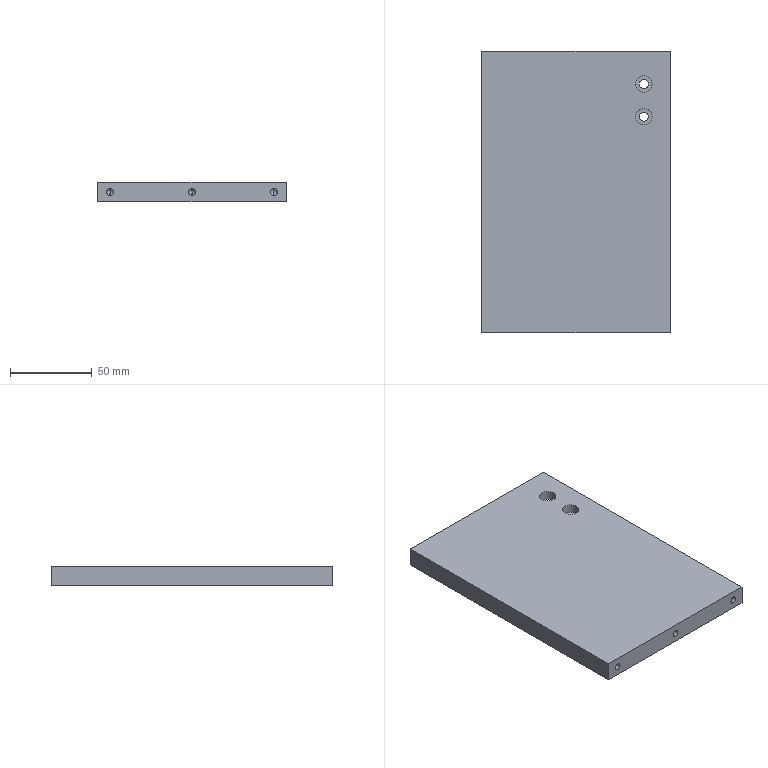Part | STEP file | PN_0002 Mount electronic clip base support plate A | 1 solid | 36 faces | box 115 x 172 x 12 mm | volume 235166 mm3 | cylinder 18 | cone 10 | plane 8 | commonest cylinder face diameters 4.2 x10 5.5 x4 10 x4